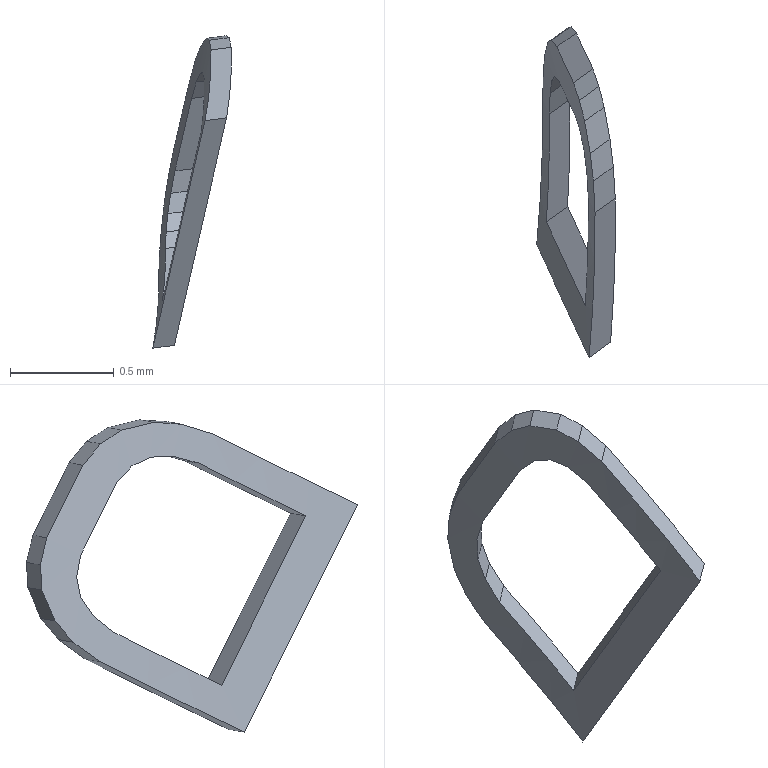Part | SolidWorks | features BaseBody 1 | 1 solid | 28 faces | box 0.379 x 1.595 x 1.505 mm | volume 0.06995 mm3 | plane 26 | cylinder 2 | commonest cylinder face diameters 16.8 x1 17 x1
STEP:
#1=CARTESIAN_POINT('',(1974.698,-243.491,991.242));
#2=VERTEX_POINT('',#1);
#3=CARTESIAN_POINT('',(1974.727,-242.792,991.583));
#4=VERTEX_POINT('',#3);
#5=CARTESIAN_POINT('',(1966.499,-243.608,993.067));
#6=DIRECTION('',(0.2015,-0.436,0.8771));
#7=DIRECTION('',(-0.7309,-0.6631,-0.1618));
#8=AXIS2_PLACEMENT_3D('',#5,#6,#7);
#9=CIRCLE('',#8,8.4);
#10=EDGE_CURVE('',#2,#4,#9,.T.);
#11=ORIENTED_EDGE('',*,*,#10,.T.);
#12=CARTESIAN_POINT('',(1974.718,-242.641,991.629));
#13=VERTEX_POINT('',#12);
#14=CARTESIAN_POINT('',(1974.727,-242.792,991.583));
#15=CARTESIAN_POINT('',(1974.724,-242.742,991.598));
#16=CARTESIAN_POINT('',(1974.722,-242.691,991.614));
#17=CARTESIAN_POINT('',(1974.718,-242.641,991.629));
#18=B_SPLINE_CURVE_WITH_KNOTS('',3,(#14,#15,#16,#17),.UNSPECIFIED.,.F.,.F.,(4,4),(0.,1.),.UNSPECIFIED.);
#19=EDGE_CURVE('',#4,#13,#18,.T.);
#20=ORIENTED_EDGE('',*,*,#19,.T.);
#21=CARTESIAN_POINT('',(1974.704,-242.508,991.638));
#22=VERTEX_POINT('',#21);
#23=CARTESIAN_POINT('',(1974.718,-242.641,991.629));
#24=CARTESIAN_POINT('',(1974.714,-242.597,991.632));
#25=CARTESIAN_POINT('',(1974.709,-242.552,991.635));
#26=CARTESIAN_POINT('',(1974.704,-242.508,991.638));
#27=B_SPLINE_CURVE_WITH_KNOTS('',3,(#23,#24,#25,#26),.UNSPECIFIED.,.F.,.F.,(4,4),(0.,1.),.UNSPECIFIED.);
#28=EDGE_CURVE('',#13,#22,#27,.T.);
#29=ORIENTED_EDGE('',*,*,#28,.T.);
#30=CARTESIAN_POINT('',(1974.676,-242.353,991.6));
#31=VERTEX_POINT('',#30);
#32=CARTESIAN_POINT('',(1974.704,-242.508,991.638));
#33=CARTESIAN_POINT('',(1974.695,-242.456,991.625));
#34=CARTESIAN_POINT('',(1974.686,-242.404,991.613));
#35=CARTESIAN_POINT('',(1974.676,-242.353,991.6));
#36=B_SPLINE_CURVE_WITH_KNOTS('',3,(#32,#33,#34,#35),.UNSPECIFIED.,.F.,.F.,(4,4),(0.,1.),.UNSPECIFIED.);
#37=EDGE_CURVE('',#22,#31,#36,.T.);
#38=ORIENTED_EDGE('',*,*,#37,.T.);
#39=CARTESIAN_POINT('',(1974.651,-242.252,991.534));
#40=VERTEX_POINT('',#39);
#41=CARTESIAN_POINT('',(1974.676,-242.353,991.6));
#42=CARTESIAN_POINT('',(1974.668,-242.319,991.578));
#43=CARTESIAN_POINT('',(1974.66,-242.286,991.556));
#44=CARTESIAN_POINT('',(1974.651,-242.252,991.534));
#45=B_SPLINE_CURVE_WITH_KNOTS('',3,(#41,#42,#43,#44),.UNSPECIFIED.,.F.,.F.,(4,4),(0.,1.),.UNSPECIFIED.);
#46=EDGE_CURVE('',#31,#40,#45,.T.);
#47=ORIENTED_EDGE('',*,*,#46,.T.);
#48=CARTESIAN_POINT('',(1974.623,-242.168,991.432));
#49=VERTEX_POINT('',#48);
#50=CARTESIAN_POINT('',(1974.651,-242.252,991.534));
#51=CARTESIAN_POINT('',(1974.642,-242.224,991.5));
#52=CARTESIAN_POINT('',(1974.632,-242.196,991.466));
#53=CARTESIAN_POINT('',(1974.623,-242.168,991.432));
#54=B_SPLINE_CURVE_WITH_KNOTS('',3,(#50,#51,#52,#53),.UNSPECIFIED.,.F.,.F.,(4,4),(0.,1.),.UNSPECIFIED.);
#55=EDGE_CURVE('',#40,#49,#54,.T.);
#56=ORIENTED_EDGE('',*,*,#55,.T.);
#57=CARTESIAN_POINT('',(1974.542,-241.994,991.082));
#58=VERTEX_POINT('',#57);
#59=CARTESIAN_POINT('',(1975.659,-244.411,995.945));
#60=DIRECTION('',(-0.2015,0.436,-0.8771));
#61=VECTOR('',#60,1000.);
#62=LINE('',#59,#61);
#63=EDGE_CURVE('',#49,#58,#62,.T.);
#64=ORIENTED_EDGE('',*,*,#63,.T.);
#65=CARTESIAN_POINT('',(1974.517,-241.963,990.951));
#66=VERTEX_POINT('',#65);
#67=CARTESIAN_POINT('',(1974.517,-241.963,990.951));
#68=CARTESIAN_POINT('',(1974.526,-241.973,990.995));
#69=CARTESIAN_POINT('',(1974.534,-241.983,991.038));
#70=CARTESIAN_POINT('',(1974.542,-241.994,991.082));
#71=B_SPLINE_CURVE_WITH_KNOTS('',3,(#67,#68,#69,#70),.UNSPECIFIED.,.F.,.F.,(4,4),(0.,1.),.UNSPECIFIED.);
#72=EDGE_CURVE('',#66,#58,#71,.T.);
#73=ORIENTED_EDGE('',*,*,#72,.F.);
#74=CARTESIAN_POINT('',(1974.5,-241.97,990.83));
#75=VERTEX_POINT('',#74);
#76=CARTESIAN_POINT('',(1974.5,-241.97,990.83));
#77=CARTESIAN_POINT('',(1974.506,-241.967,990.871));
#78=CARTESIAN_POINT('',(1974.512,-241.965,990.911));
#79=CARTESIAN_POINT('',(1974.517,-241.963,990.951));
#80=B_SPLINE_CURVE_WITH_KNOTS('',3,(#76,#77,#78,#79),.UNSPECIFIED.,.F.,.F.,(4,4),(0.,1.),.UNSPECIFIED.);
#81=EDGE_CURVE('',#75,#66,#80,.T.);
#82=ORIENTED_EDGE('',*,*,#81,.F.);
#83=CARTESIAN_POINT('',(1974.484,-242.032,990.682));
#84=VERTEX_POINT('',#83);
#85=CARTESIAN_POINT('',(1974.484,-242.032,990.682));
#86=CARTESIAN_POINT('',(1974.489,-242.012,990.731));
#87=CARTESIAN_POINT('',(1974.495,-241.991,990.781));
#88=CARTESIAN_POINT('',(1974.5,-241.97,990.83));
#89=B_SPLINE_CURVE_WITH_KNOTS('',3,(#85,#86,#87,#88),.UNSPECIFIED.,.F.,.F.,(4,4),(0.,1.),.UNSPECIFIED.);
#90=EDGE_CURVE('',#84,#75,#89,.T.);
#91=ORIENTED_EDGE('',*,*,#90,.F.);
#92=CARTESIAN_POINT('',(1974.477,-242.119,990.579));
#93=VERTEX_POINT('',#92);
#94=CARTESIAN_POINT('',(1974.477,-242.119,990.579));
#95=CARTESIAN_POINT('',(1974.48,-242.09,990.613));
#96=CARTESIAN_POINT('',(1974.482,-242.061,990.647));
#97=CARTESIAN_POINT('',(1974.484,-242.032,990.682));
#98=B_SPLINE_CURVE_WITH_KNOTS('',3,(#94,#95,#96,#97),.UNSPECIFIED.,.F.,.F.,(4,4),(0.,1.),.UNSPECIFIED.);
#99=EDGE_CURVE('',#93,#84,#98,.T.);
#100=ORIENTED_EDGE('',*,*,#99,.F.);
#101=CARTESIAN_POINT('',(1974.475,-242.247,990.486));
#102=VERTEX_POINT('',#101);
#103=CARTESIAN_POINT('',(1974.475,-242.247,990.486));
#104=CARTESIAN_POINT('',(1974.476,-242.204,990.517));
#105=CARTESIAN_POINT('',(1974.477,-242.162,990.548));
#106=CARTESIAN_POINT('',(1974.477,-242.119,990.579));
#107=B_SPLINE_CURVE_WITH_KNOTS('',3,(#103,#104,#105,#106),.UNSPECIFIED.,.F.,.F.,(4,4),(0.,1.),.UNSPECIFIED.);
#108=EDGE_CURVE('',#102,#93,#107,.T.);
#109=ORIENTED_EDGE('',*,*,#108,.F.);
#110=CARTESIAN_POINT('',(1974.446,-242.945,990.146));
#111=VERTEX_POINT('',#110);
#112=CARTESIAN_POINT('',(1966.247,-243.063,991.97));
#113=DIRECTION('',(-0.2015,0.436,-0.8771));
#114=DIRECTION('',(-0.7309,-0.6631,-0.1618));
#115=AXIS2_PLACEMENT_3D('',#112,#113,#114);
#116=CIRCLE('',#115,8.4);
#117=EDGE_CURVE('',#102,#111,#116,.T.);
#118=ORIENTED_EDGE('',*,*,#117,.T.);
#119=CARTESIAN_POINT('',(1975.649,-245.549,995.382));
#120=DIRECTION('',(0.2015,-0.436,0.8771));
#121=VECTOR('',#120,1000.);
#122=LINE('',#119,#121);
#123=EDGE_CURVE('',#111,#2,#122,.T.);
#124=ORIENTED_EDGE('',*,*,#123,.T.);
#125=EDGE_LOOP('',(#11,#20,#29,#38,#47,#56,#64,#73,#82,#91,#100,#109,#118,#124));
#126=FACE_OUTER_BOUND('',#125,.T.);
#127=CARTESIAN_POINT('',(1974.507,-242.317,990.626));
#128=VERTEX_POINT('',#127);
#129=CARTESIAN_POINT('',(1974.51,-242.217,990.705));
#130=VERTEX_POINT('',#129);
#131=CARTESIAN_POINT('',(1974.507,-242.317,990.626));
#132=CARTESIAN_POINT('',(1974.508,-242.283,990.652));
#133=CARTESIAN_POINT('',(1974.509,-242.25,990.679));
#134=CARTESIAN_POINT('',(1974.51,-242.217,990.705));
#135=B_SPLINE_CURVE_WITH_KNOTS('',3,(#131,#132,#133,#134),.UNSPECIFIED.,.F.,.F.,(4,4),(0.,1.),.UNSPECIFIED.);
#136=EDGE_CURVE('',#128,#130,#135,.T.);
#137=ORIENTED_EDGE('',*,*,#136,.T.);
#138=CARTESIAN_POINT('',(1974.518,-242.157,990.794));
#139=VERTEX_POINT('',#138);
#140=CARTESIAN_POINT('',(1974.51,-242.217,990.705));
#141=CARTESIAN_POINT('',(1974.513,-242.197,990.735));
#142=CARTESIAN_POINT('',(1974.516,-242.177,990.764));
#143=CARTESIAN_POINT('',(1974.518,-242.157,990.794));
#144=B_SPLINE_CURVE_WITH_KNOTS('',3,(#140,#141,#142,#143),.UNSPECIFIED.,.F.,.F.,(4,4),(0.,1.),.UNSPECIFIED.);
#145=EDGE_CURVE('',#130,#139,#144,.T.);
#146=ORIENTED_EDGE('',*,*,#145,.T.);
#147=CARTESIAN_POINT('',(1974.532,-242.137,990.892));
#148=VERTEX_POINT('',#147);
#149=CARTESIAN_POINT('',(1974.518,-242.157,990.794));
#150=CARTESIAN_POINT('',(1974.523,-242.15,990.826));
#151=CARTESIAN_POINT('',(1974.528,-242.143,990.859));
#152=CARTESIAN_POINT('',(1974.532,-242.137,990.892));
#153=B_SPLINE_CURVE_WITH_KNOTS('',3,(#149,#150,#151,#152),.UNSPECIFIED.,.F.,.F.,(4,4),(0.,1.),.UNSPECIFIED.);
#154=EDGE_CURVE('',#139,#148,#153,.T.);
#155=ORIENTED_EDGE('',*,*,#154,.T.);
#156=CARTESIAN_POINT('',(1974.552,-242.156,990.999));
#157=VERTEX_POINT('',#156);
#158=CARTESIAN_POINT('',(1974.532,-242.137,990.892));
#159=CARTESIAN_POINT('',(1974.539,-242.143,990.927));
#160=CARTESIAN_POINT('',(1974.546,-242.15,990.963));
#161=CARTESIAN_POINT('',(1974.552,-242.156,990.999));
#162=B_SPLINE_CURVE_WITH_KNOTS('',3,(#158,#159,#160,#161),.UNSPECIFIED.,.F.,.F.,(4,4),(0.,1.),.UNSPECIFIED.);
#163=EDGE_CURVE('',#148,#157,#162,.T.);
#164=ORIENTED_EDGE('',*,*,#163,.T.);
#165=CARTESIAN_POINT('',(1974.633,-242.33,991.349));
#166=VERTEX_POINT('',#165);
#167=CARTESIAN_POINT('',(1975.669,-244.574,995.862));
#168=DIRECTION('',(-0.2015,0.436,-0.8771));
#169=VECTOR('',#168,1000.);
#170=LINE('',#167,#169);
#171=EDGE_CURVE('',#166,#157,#170,.T.);
#172=ORIENTED_EDGE('',*,*,#171,.F.);
#173=CARTESIAN_POINT('',(1974.655,-242.404,991.428));
#174=VERTEX_POINT('',#173);
#175=CARTESIAN_POINT('',(1974.655,-242.404,991.428));
#176=CARTESIAN_POINT('',(1974.648,-242.379,991.402));
#177=CARTESIAN_POINT('',(1974.64,-242.354,991.375));
#178=CARTESIAN_POINT('',(1974.633,-242.33,991.349));
#179=B_SPLINE_CURVE_WITH_KNOTS('',3,(#175,#176,#177,#178),.UNSPECIFIED.,.F.,.F.,(4,4),(0.,1.),.UNSPECIFIED.);
#180=EDGE_CURVE('',#174,#166,#179,.T.);
#181=ORIENTED_EDGE('',*,*,#180,.F.);
#182=CARTESIAN_POINT('',(1974.674,-242.493,991.47));
#183=VERTEX_POINT('',#182);
#184=CARTESIAN_POINT('',(1974.674,-242.493,991.47));
#185=CARTESIAN_POINT('',(1974.668,-242.463,991.456));
#186=CARTESIAN_POINT('',(1974.662,-242.433,991.442));
#187=CARTESIAN_POINT('',(1974.655,-242.404,991.428));
#188=B_SPLINE_CURVE_WITH_KNOTS('',3,(#184,#185,#186,#187),.UNSPECIFIED.,.F.,.F.,(4,4),(0.,1.),.UNSPECIFIED.);
#189=EDGE_CURVE('',#183,#174,#188,.T.);
#190=ORIENTED_EDGE('',*,*,#189,.F.);
#191=CARTESIAN_POINT('',(1974.687,-242.599,991.475));
#192=VERTEX_POINT('',#191);
#193=CARTESIAN_POINT('',(1974.687,-242.599,991.475));
#194=CARTESIAN_POINT('',(1974.683,-242.564,991.474));
#195=CARTESIAN_POINT('',(1974.678,-242.529,991.472));
#196=CARTESIAN_POINT('',(1974.674,-242.493,991.47));
#197=B_SPLINE_CURVE_WITH_KNOTS('',3,(#193,#194,#195,#196),.UNSPECIFIED.,.F.,.F.,(4,4),(0.,1.),.UNSPECIFIED.);
#198=EDGE_CURVE('',#192,#183,#197,.T.);
#199=ORIENTED_EDGE('',*,*,#198,.F.);
#200=CARTESIAN_POINT('',(1974.694,-242.722,991.443));
#201=VERTEX_POINT('',#200);
#202=CARTESIAN_POINT('',(1974.694,-242.722,991.443));
#203=CARTESIAN_POINT('',(1974.692,-242.681,991.453));
#204=CARTESIAN_POINT('',(1974.69,-242.64,991.464));
#205=CARTESIAN_POINT('',(1974.687,-242.599,991.475));
#206=B_SPLINE_CURVE_WITH_KNOTS('',3,(#202,#203,#204,#205),.UNSPECIFIED.,.F.,.F.,(4,4),(0.,1.),.UNSPECIFIED.);
#207=EDGE_CURVE('',#201,#192,#206,.T.);
#208=ORIENTED_EDGE('',*,*,#207,.F.);
#209=CARTESIAN_POINT('',(1974.68,-243.241,991.188));
#210=VERTEX_POINT('',#209);
#211=CARTESIAN_POINT('',(1966.467,-243.538,992.927));
#212=DIRECTION('',(0.2015,-0.436,0.8771));
#213=DIRECTION('',(-0.7309,-0.6631,-0.1618));
#214=AXIS2_PLACEMENT_3D('',#211,#212,#213);
#215=CIRCLE('',#214,8.4);
#216=EDGE_CURVE('',#210,#201,#215,.T.);
#217=ORIENTED_EDGE('',*,*,#216,.F.);
#218=CARTESIAN_POINT('',(1974.492,-242.835,990.372));
#219=VERTEX_POINT('',#218);
#220=CARTESIAN_POINT('',(1975.663,-245.369,995.468));
#221=DIRECTION('',(0.2015,-0.436,0.8771));
#222=VECTOR('',#221,1000.);
#223=LINE('',#220,#222);
#224=EDGE_CURVE('',#219,#210,#223,.T.);
#225=ORIENTED_EDGE('',*,*,#224,.F.);
#226=CARTESIAN_POINT('',(1966.279,-243.133,992.11));
#227=DIRECTION('',(-0.2015,0.436,-0.8771));
#228=DIRECTION('',(-0.7309,-0.6631,-0.1618));
#229=AXIS2_PLACEMENT_3D('',#226,#227,#228);
#230=CIRCLE('',#229,8.4);
#231=EDGE_CURVE('',#128,#219,#230,.T.);
#232=ORIENTED_EDGE('',*,*,#231,.F.);
#233=EDGE_LOOP('',(#137,#146,#155,#164,#172,#181,#190,#199,#208,#217,#225,#232));
#234=FACE_BOUND('',#233,.T.);
#235=CARTESIAN_POINT('',(1967.45,-245.666,997.207));
#236=DIRECTION('',(0.2015,-0.436,0.8771));
#237=DIRECTION('',(-0.7309,-0.6631,-0.1618));
#238=AXIS2_PLACEMENT_3D('',#235,#236,#237);
#239=CYLINDRICAL_SURFACE('',#238,8.4);
#240=ADVANCED_FACE('',(#126,#234),#239,.F.);
#241=CARTESIAN_POINT('',(1974.802,-243.416,991.255));
#242=VERTEX_POINT('',#241);
#243=CARTESIAN_POINT('',(1974.75,-243.453,991.248));
#244=DIRECTION('',(-0.8088,-0.5792,-0.1022));
#245=VECTOR('',#244,1000.);
#246=LINE('',#243,#245);
#247=EDGE_CURVE('',#242,#2,#246,.T.);
#248=ORIENTED_EDGE('',*,*,#247,.T.);
#249=ORIENTED_EDGE('',*,*,#123,.F.);
#250=CARTESIAN_POINT('',(1974.55,-242.871,990.159));
#251=VERTEX_POINT('',#250);
#252=CARTESIAN_POINT('',(1974.498,-242.908,990.152));
#253=DIRECTION('',(-0.8088,-0.5792,-0.1022));
#254=VECTOR('',#253,1000.);
#255=LINE('',#252,#254);
#256=EDGE_CURVE('',#251,#111,#255,.T.);
#257=ORIENTED_EDGE('',*,*,#256,.F.);
#258=CARTESIAN_POINT('',(1974.676,-243.144,990.707));
#259=DIRECTION('',(0.2015,-0.436,0.8771));
#260=VECTOR('',#259,1000.);
#261=LINE('',#258,#260);
#262=EDGE_CURVE('',#251,#242,#261,.T.);
#263=ORIENTED_EDGE('',*,*,#262,.T.);
#264=EDGE_LOOP('',(#248,#249,#257,#263));
#265=FACE_OUTER_BOUND('',#264,.T.);
#266=CARTESIAN_POINT('',(1981.31,-238.029,991.013));
#267=DIRECTION('',(0.5526,-0.6888,-0.4693));
#268=DIRECTION('',(-0.2015,0.436,-0.8771));
#269=AXIS2_PLACEMENT_3D('',#266,#267,#268);
#270=PLANE('',#269);
#271=ADVANCED_FACE('',(#265),#270,.T.);
#272=ORIENTED_EDGE('',*,*,#256,.T.);
#273=ORIENTED_EDGE('',*,*,#117,.F.);
#274=CARTESIAN_POINT('',(1974.572,-242.177,990.498));
#275=VERTEX_POINT('',#274);
#276=CARTESIAN_POINT('',(1974.523,-242.212,990.492));
#277=DIRECTION('',(-0.8088,-0.5792,-0.1022));
#278=VECTOR('',#277,1000.);
#279=LINE('',#276,#278);
#280=EDGE_CURVE('',#275,#102,#279,.T.);
#281=ORIENTED_EDGE('',*,*,#280,.F.);
#282=CARTESIAN_POINT('',(1966.247,-243.063,991.97));
#283=DIRECTION('',(-0.2015,0.436,-0.8771));
#284=DIRECTION('',(-0.7309,-0.6631,-0.1618));
#285=AXIS2_PLACEMENT_3D('',#282,#283,#284);
#286=CIRCLE('',#285,8.5);
#287=EDGE_CURVE('',#275,#251,#286,.T.);
#288=ORIENTED_EDGE('',*,*,#287,.T.);
#289=EDGE_LOOP('',(#272,#273,#281,#288));
#290=FACE_OUTER_BOUND('',#289,.T.);
#291=CARTESIAN_POINT('',(1981.656,-238.46,990.719));
#292=DIRECTION('',(-0.2015,0.436,-0.8771));
#293=DIRECTION('',(-0.5526,0.6888,0.4693));
#294=AXIS2_PLACEMENT_3D('',#291,#292,#293);
#295=PLANE('',#294);
#296=ADVANCED_FACE('',(#290),#295,.T.);
#297=ORIENTED_EDGE('',*,*,#280,.T.);
#298=ORIENTED_EDGE('',*,*,#108,.T.);
#299=CARTESIAN_POINT('',(1974.573,-242.051,990.591));
#300=VERTEX_POINT('',#299);
#301=CARTESIAN_POINT('',(1974.525,-242.085,990.585));
#302=DIRECTION('',(-0.8088,-0.5792,-0.1022));
#303=VECTOR('',#302,1000.);
#304=LINE('',#301,#303);
#305=EDGE_CURVE('',#300,#93,#304,.T.);
#306=ORIENTED_EDGE('',*,*,#305,.F.);
#307=CARTESIAN_POINT('',(1974.572,-242.177,990.498));
#308=CARTESIAN_POINT('',(1974.572,-242.152,990.517));
#309=CARTESIAN_POINT('',(1974.573,-242.127,990.536));
#310=CARTESIAN_POINT('',(1974.573,-242.101,990.554));
#311=CARTESIAN_POINT('',(1974.573,-242.076,990.573));
#312=CARTESIAN_POINT('',(1974.573,-242.051,990.591));
#313=B_SPLINE_CURVE_WITH_KNOTS('',5,(#307,#308,#309,#310,#311,#312),.UNSPECIFIED.,.F.,.F.,(6,6),(0.,1.),.UNSPECIFIED.);
#314=EDGE_CURVE('',#275,#300,#313,.T.);
#315=ORIENTED_EDGE('',*,*,#314,.F.);
#316=EDGE_LOOP('',(#297,#298,#306,#315));
#317=FACE_OUTER_BOUND('',#316,.T.);
#318=CARTESIAN_POINT('',(1980.898,-237.521,991.391));
#319=DIRECTION('',(-0.308,0.5651,-0.7654));
#320=DIRECTION('',(-0.5011,0.5876,0.6354));
#321=AXIS2_PLACEMENT_3D('',#318,#319,#320);
#322=PLANE('',#321);
#323=ADVANCED_FACE('',(#317),#322,.T.);
#324=ORIENTED_EDGE('',*,*,#305,.T.);
#325=ORIENTED_EDGE('',*,*,#99,.T.);
#326=CARTESIAN_POINT('',(1974.579,-241.964,990.694));
#327=VERTEX_POINT('',#326);
#328=CARTESIAN_POINT('',(1974.531,-241.998,990.688));
#329=DIRECTION('',(-0.8088,-0.5792,-0.1022));
#330=VECTOR('',#329,1000.);
#331=LINE('',#328,#330);
#332=EDGE_CURVE('',#327,#84,#331,.T.);
#333=ORIENTED_EDGE('',*,*,#332,.F.);
#334=CARTESIAN_POINT('',(1974.573,-242.051,990.591));
#335=CARTESIAN_POINT('',(1974.575,-242.033,990.612));
#336=CARTESIAN_POINT('',(1974.576,-242.016,990.632));
#337=CARTESIAN_POINT('',(1974.577,-241.999,990.653));
#338=CARTESIAN_POINT('',(1974.578,-241.982,990.673));
#339=CARTESIAN_POINT('',(1974.579,-241.964,990.694));
#340=B_SPLINE_CURVE_WITH_KNOTS('',5,(#334,#335,#336,#337,#338,#339),.UNSPECIFIED.,.F.,.F.,(6,6),(0.,1.),.UNSPECIFIED.);
#341=EDGE_CURVE('',#300,#327,#340,.T.);
#342=ORIENTED_EDGE('',*,*,#341,.F.);
#343=EDGE_LOOP('',(#324,#325,#333,#342));
#344=FACE_OUTER_BOUND('',#343,.T.);
#345=CARTESIAN_POINT('',(1980.851,-237.472,991.486));
#346=DIRECTION('',(-0.4307,0.7016,-0.5677));
#347=DIRECTION('',(-0.4005,0.4151,0.8169));
#348=AXIS2_PLACEMENT_3D('',#345,#346,#347);
#349=PLANE('',#348);
#350=ADVANCED_FACE('',(#344),#349,.T.);
#351=ORIENTED_EDGE('',*,*,#332,.T.);
#352=ORIENTED_EDGE('',*,*,#90,.T.);
#353=CARTESIAN_POINT('',(1974.594,-241.903,990.842));
#354=VERTEX_POINT('',#353);
#355=CARTESIAN_POINT('',(1974.547,-241.936,990.836));
#356=DIRECTION('',(-0.8088,-0.5792,-0.1022));
#357=VECTOR('',#356,1000.);
#358=LINE('',#355,#357);
#359=EDGE_CURVE('',#354,#75,#358,.T.);
#360=ORIENTED_EDGE('',*,*,#359,.F.);
#361=CARTESIAN_POINT('',(1974.579,-241.964,990.694));
#362=CARTESIAN_POINT('',(1974.582,-241.952,990.723));
#363=CARTESIAN_POINT('',(1974.585,-241.939,990.753));
#364=CARTESIAN_POINT('',(1974.588,-241.927,990.783));
#365=CARTESIAN_POINT('',(1974.591,-241.915,990.813));
#366=CARTESIAN_POINT('',(1974.594,-241.903,990.842));
#367=B_SPLINE_CURVE_WITH_KNOTS('',5,(#361,#362,#363,#364,#365,#366),.UNSPECIFIED.,.F.,.F.,(6,6),(0.,1.),.UNSPECIFIED.);
#368=EDGE_CURVE('',#327,#354,#367,.T.);
#369=ORIENTED_EDGE('',*,*,#368,.F.);
#370=EDGE_LOOP('',(#351,#352,#360,#369));
#371=FACE_OUTER_BOUND('',#370,.T.);
#372=CARTESIAN_POINT('',(1980.815,-237.447,991.628));
#373=DIRECTION('',(-0.5358,0.7972,-0.2783));
#374=DIRECTION('',(-0.2426,0.1703,0.955));
#375=AXIS2_PLACEMENT_3D('',#372,#373,#374);
#376=PLANE('',#375);
#377=ADVANCED_FACE('',(#371),#376,.T.);
#378=ORIENTED_EDGE('',*,*,#359,.T.);
#379=ORIENTED_EDGE('',*,*,#81,.T.);
#380=CARTESIAN_POINT('',(1974.611,-241.895,990.963));
#381=VERTEX_POINT('',#380);
#382=CARTESIAN_POINT('',(1974.564,-241.929,990.957));
#383=DIRECTION('',(-0.8088,-0.5792,-0.1022));
#384=VECTOR('',#383,1000.);
#385=LINE('',#382,#384);
#386=EDGE_CURVE('',#381,#66,#385,.T.);
#387=ORIENTED_EDGE('',*,*,#386,.F.);
#388=CARTESIAN_POINT('',(1974.594,-241.903,990.842));
#389=CARTESIAN_POINT('',(1974.597,-241.901,990.866));
#390=CARTESIAN_POINT('',(1974.601,-241.9,990.891));
#391=CARTESIAN_POINT('',(1974.604,-241.898,990.915));
#392=CARTESIAN_POINT('',(1974.608,-241.897,990.939));
#393=CARTESIAN_POINT('',(1974.611,-241.895,990.963));
#394=B_SPLINE_CURVE_WITH_KNOTS('',5,(#388,#389,#390,#391,#392,#393),.UNSPECIFIED.,.F.,.F.,(6,6),(0.,1.),.UNSPECIFIED.);
#395=EDGE_CURVE('',#354,#381,#394,.T.);
#396=ORIENTED_EDGE('',*,*,#395,.F.);
#397=EDGE_LOOP('',(#378,#379,#387,#396));
#398=FACE_OUTER_BOUND('',#397,.T.);
#399=CARTESIAN_POINT('',(1980.808,-237.457,991.746));
#400=DIRECTION('',(-0.5849,0.8103,0.03586));
#401=DIRECTION('',(-0.06203,-0.08877,0.9941));
#402=AXIS2_PLACEMENT_3D('',#399,#400,#401);
#403=PLANE('',#402);
#404=ADVANCED_FACE('',(#398),#403,.T.);
#405=ORIENTED_EDGE('',*,*,#386,.T.);
#406=ORIENTED_EDGE('',*,*,#72,.T.);
#407=CARTESIAN_POINT('',(1974.636,-241.927,991.094));
#408=VERTEX_POINT('',#407);
#409=CARTESIAN_POINT('',(1974.589,-241.96,991.088));
#410=DIRECTION('',(-0.8088,-0.5792,-0.1022));
#411=VECTOR('',#410,1000.);
#412=LINE('',#409,#411);
#413=EDGE_CURVE('',#408,#58,#412,.T.);
#414=ORIENTED_EDGE('',*,*,#413,.F.);
#415=CARTESIAN_POINT('',(1974.611,-241.895,990.963));
#416=CARTESIAN_POINT('',(1974.616,-241.902,990.989));
#417=CARTESIAN_POINT('',(1974.621,-241.908,991.015));
#418=CARTESIAN_POINT('',(1974.626,-241.914,991.041));
#419=CARTESIAN_POINT('',(1974.631,-241.92,991.068));
#420=CARTESIAN_POINT('',(1974.636,-241.927,991.094));
#421=B_SPLINE_CURVE_WITH_KNOTS('',5,(#415,#416,#417,#418,#419,#420),.UNSPECIFIED.,.F.,.F.,(6,6),(0.,1.),.UNSPECIFIED.);
#422=EDGE_CURVE('',#381,#408,#421,.T.);
#423=ORIENTED_EDGE('',*,*,#422,.F.);
#424=EDGE_LOOP('',(#405,#406,#414,#423));
#425=FACE_OUTER_BOUND('',#424,.T.);
#426=CARTESIAN_POINT('',(1980.82,-237.497,991.875));
#427=DIRECTION('',(-0.581,0.7597,0.292));
#428=DIRECTION('',(0.09152,-0.2955,0.9509));
#429=AXIS2_PLACEMENT_3D('',#426,#427,#428);
#430=PLANE('',#429);
#431=ADVANCED_FACE('',(#425),#430,.T.);
#432=ORIENTED_EDGE('',*,*,#413,.T.);
#433=ORIENTED_EDGE('',*,*,#63,.F.);
#434=CARTESIAN_POINT('',(1974.716,-242.1,991.443));
#435=VERTEX_POINT('',#434);
#436=CARTESIAN_POINT('',(1974.669,-242.134,991.438));
#437=DIRECTION('',(-0.8088,-0.5792,-0.1022));
#438=VECTOR('',#437,1000.);
#439=LINE('',#436,#438);
#440=EDGE_CURVE('',#435,#49,#439,.T.);
#441=ORIENTED_EDGE('',*,*,#440,.F.);
#442=CARTESIAN_POINT('',(1974.676,-242.014,991.269));
#443=DIRECTION('',(-0.2015,0.436,-0.8771));
#444=VECTOR('',#443,1000.);
#445=LINE('',#442,#444);
#446=EDGE_CURVE('',#435,#408,#445,.T.);
#447=ORIENTED_EDGE('',*,*,#446,.T.);
#448=EDGE_LOOP('',(#432,#433,#441,#447));
#449=FACE_OUTER_BOUND('',#448,.T.);
#450=CARTESIAN_POINT('',(1980.901,-237.671,992.225));
#451=DIRECTION('',(-0.5526,0.6888,0.4693));
#452=DIRECTION('',(0.2015,-0.436,0.8771));
#453=AXIS2_PLACEMENT_3D('',#450,#451,#452);
#454=PLANE('',#453);
#455=ADVANCED_FACE('',(#449),#454,.T.);
#456=ORIENTED_EDGE('',*,*,#440,.T.);
#457=ORIENTED_EDGE('',*,*,#55,.F.);
#458=CARTESIAN_POINT('',(1974.745,-242.185,991.546));
#459=VERTEX_POINT('',#458);
#460=CARTESIAN_POINT('',(1974.698,-242.219,991.54));
#461=DIRECTION('',(-0.8088,-0.5792,-0.1022));
#462=VECTOR('',#461,1000.);
#463=LINE('',#460,#462);
#464=EDGE_CURVE('',#459,#40,#463,.T.);
#465=ORIENTED_EDGE('',*,*,#464,.F.);
#466=CARTESIAN_POINT('',(1974.745,-242.185,991.546));
#467=CARTESIAN_POINT('',(1974.739,-242.168,991.526));
#468=CARTESIAN_POINT('',(1974.734,-242.151,991.505));
#469=CARTESIAN_POINT('',(1974.728,-242.134,991.485));
#470=CARTESIAN_POINT('',(1974.722,-242.117,991.464));
#471=CARTESIAN_POINT('',(1974.716,-242.1,991.443));
#472=B_SPLINE_CURVE_WITH_KNOTS('',5,(#466,#467,#468,#469,#470,#471),.UNSPECIFIED.,.F.,.F.,(6,6),(0.,1.),.UNSPECIFIED.);
#473=EDGE_CURVE('',#459,#435,#472,.T.);
#474=ORIENTED_EDGE('',*,*,#473,.T.);
#475=EDGE_LOOP('',(#456,#457,#465,#474));
#476=FACE_OUTER_BOUND('',#475,.T.);
#477=CARTESIAN_POINT('',(1980.942,-237.747,992.329));
#478=DIRECTION('',(-0.5035,0.5921,0.6292));
#479=DIRECTION('',(0.3039,-0.5603,0.7705));
#480=AXIS2_PLACEMENT_3D('',#477,#478,#479);
#481=PLANE('',#480);
#482=ADVANCED_FACE('',(#476),#481,.T.);
#483=ORIENTED_EDGE('',*,*,#464,.T.);
#484=ORIENTED_EDGE('',*,*,#46,.F.);
#485=CARTESIAN_POINT('',(1974.771,-242.285,991.612));
#486=VERTEX_POINT('',#485);
#487=CARTESIAN_POINT('',(1974.723,-242.319,991.606));
#488=DIRECTION('',(-0.8088,-0.5792,-0.1022));
#489=VECTOR('',#488,1000.);
#490=LINE('',#487,#489);
#491=EDGE_CURVE('',#486,#31,#490,.T.);
#492=ORIENTED_EDGE('',*,*,#491,.F.);
#493=CARTESIAN_POINT('',(1974.771,-242.285,991.612));
#494=CARTESIAN_POINT('',(1974.766,-242.265,991.599));
#495=CARTESIAN_POINT('',(1974.761,-242.245,991.586));
#496=CARTESIAN_POINT('',(1974.755,-242.225,991.573));
#497=CARTESIAN_POINT('',(1974.75,-242.205,991.56));
#498=CARTESIAN_POINT('',(1974.745,-242.185,991.546));
#499=B_SPLINE_CURVE_WITH_KNOTS('',5,(#493,#494,#495,#496,#497,#498),.UNSPECIFIED.,.F.,.F.,(6,6),(0.,1.),.UNSPECIFIED.);
#500=EDGE_CURVE('',#486,#459,#499,.T.);
#501=ORIENTED_EDGE('',*,*,#500,.T.);
#502=EDGE_LOOP('',(#483,#484,#492,#501));
#503=FACE_OUTER_BOUND('',#502,.T.);
#504=CARTESIAN_POINT('',(1980.992,-237.83,992.398));
#505=DIRECTION('',(-0.4077,0.4269,0.8072));
#506=DIRECTION('',(0.4239,-0.6945,0.5814));
#507=AXIS2_PLACEMENT_3D('',#504,#505,#506);
#508=PLANE('',#507);
#509=ADVANCED_FACE('',(#503),#508,.T.);
#510=ORIENTED_EDGE('',*,*,#491,.T.);
#511=ORIENTED_EDGE('',*,*,#37,.F.);
#512=CARTESIAN_POINT('',(1974.799,-242.44,991.65));
#513=VERTEX_POINT('',#512);
#514=CARTESIAN_POINT('',(1974.751,-242.474,991.644));
#515=DIRECTION('',(-0.8088,-0.5792,-0.1022));
#516=VECTOR('',#515,1000.);
#517=LINE('',#514,#516);
#518=EDGE_CURVE('',#513,#22,#517,.T.);
#519=ORIENTED_EDGE('',*,*,#518,.F.);
#520=CARTESIAN_POINT('',(1974.799,-242.44,991.65));
#521=CARTESIAN_POINT('',(1974.793,-242.409,991.643));
#522=CARTESIAN_POINT('',(1974.788,-242.378,991.635));
#523=CARTESIAN_POINT('',(1974.782,-242.347,991.627));
#524=CARTESIAN_POINT('',(1974.776,-242.316,991.62));
#525=CARTESIAN_POINT('',(1974.771,-242.285,991.612));
#526=B_SPLINE_CURVE_WITH_KNOTS('',5,(#520,#521,#522,#523,#524,#525),.UNSPECIFIED.,.F.,.F.,(6,6),(0.,1.),.UNSPECIFIED.);
#527=EDGE_CURVE('',#513,#486,#526,.T.);
#528=ORIENTED_EDGE('',*,*,#527,.T.);
#529=EDGE_LOOP('',(#510,#511,#519,#528));
#530=FACE_OUTER_BOUND('',#529,.T.);
#531=CARTESIAN_POINT('',(1981.071,-237.948,992.443));
#532=DIRECTION('',(-0.2539,0.1871,0.949));
#533=DIRECTION('',(0.5305,-0.7934,0.2983));
#534=AXIS2_PLACEMENT_3D('',#531,#532,#533);
#535=PLANE('',#534);
#536=ADVANCED_FACE('',(#530),#535,.T.);
#537=ORIENTED_EDGE('',*,*,#518,.T.);
#538=ORIENTED_EDGE('',*,*,#28,.F.);
#539=CARTESIAN_POINT('',(1974.814,-242.572,991.641));
#540=VERTEX_POINT('',#539);
#541=CARTESIAN_POINT('',(1974.766,-242.607,991.635));
#542=DIRECTION('',(-0.8088,-0.5792,-0.1022));
#543=VECTOR('',#542,1000.);
#544=LINE('',#541,#543);
#545=EDGE_CURVE('',#540,#13,#544,.T.);
#546=ORIENTED_EDGE('',*,*,#545,.F.);
#547=CARTESIAN_POINT('',(1974.814,-242.572,991.641));
#548=CARTESIAN_POINT('',(1974.811,-242.546,991.643));
#549=CARTESIAN_POINT('',(1974.808,-242.519,991.645));
#550=CARTESIAN_POINT('',(1974.805,-242.493,991.647));
#551=CARTESIAN_POINT('',(1974.802,-242.466,991.648));
#552=CARTESIAN_POINT('',(1974.799,-242.44,991.65));
#553=B_SPLINE_CURVE_WITH_KNOTS('',5,(#547,#548,#549,#550,#551,#552),.UNSPECIFIED.,.F.,.F.,(6,6),(0.,1.),.UNSPECIFIED.);
#554=EDGE_CURVE('',#540,#513,#553,.T.);
#555=ORIENTED_EDGE('',*,*,#554,.T.);
#556=EDGE_LOOP('',(#537,#538,#546,#555));
#557=FACE_OUTER_BOUND('',#556,.T.);
#558=CARTESIAN_POINT('',(1981.139,-238.043,992.44));
#559=DIRECTION('',(-0.07187,-0.07511,0.9946));
#560=DIRECTION('',(0.5837,-0.8117,-0.01912));
#561=AXIS2_PLACEMENT_3D('',#558,#559,#560);
#562=PLANE('',#561);
#563=ADVANCED_FACE('',(#557),#562,.T.);
#564=ORIENTED_EDGE('',*,*,#545,.T.);
#565=ORIENTED_EDGE('',*,*,#19,.F.);
#566=CARTESIAN_POINT('',(1974.824,-242.722,991.595));
#567=VERTEX_POINT('',#566);
#568=CARTESIAN_POINT('',(1974.775,-242.757,991.589));
#569=DIRECTION('',(-0.8088,-0.5792,-0.1022));
#570=VECTOR('',#569,1000.);
#571=LINE('',#568,#570);
#572=EDGE_CURVE('',#567,#4,#571,.T.);
#573=ORIENTED_EDGE('',*,*,#572,.F.);
#574=CARTESIAN_POINT('',(1974.824,-242.722,991.595));
#575=CARTESIAN_POINT('',(1974.822,-242.692,991.604));
#576=CARTESIAN_POINT('',(1974.82,-242.662,991.613));
#577=CARTESIAN_POINT('',(1974.819,-242.632,991.623));
#578=CARTESIAN_POINT('',(1974.817,-242.602,991.632));
#579=CARTESIAN_POINT('',(1974.814,-242.572,991.641));
#580=B_SPLINE_CURVE_WITH_KNOTS('',5,(#574,#575,#576,#577,#578,#579),.UNSPECIFIED.,.F.,.F.,(6,6),(0.,1.),.UNSPECIFIED.);
#581=EDGE_CURVE('',#567,#540,#580,.T.);
#582=ORIENTED_EDGE('',*,*,#581,.T.);
#583=EDGE_LOOP('',(#564,#565,#573,#582));
#584=FACE_OUTER_BOUND('',#583,.T.);
#585=CARTESIAN_POINT('',(1981.217,-238.144,992.403));
#586=DIRECTION('',(0.08681,-0.2894,0.9533));
#587=DIRECTION('',(0.5817,-0.7621,-0.2843));
#588=AXIS2_PLACEMENT_3D('',#585,#586,#587);
#589=PLANE('',#588);
#590=ADVANCED_FACE('',(#584),#589,.T.);
#591=ORIENTED_EDGE('',*,*,#572,.T.);
#592=ORIENTED_EDGE('',*,*,#10,.F.);
#593=ORIENTED_EDGE('',*,*,#247,.F.);
#594=CARTESIAN_POINT('',(1966.499,-243.608,993.067));
#595=DIRECTION('',(0.2015,-0.436,0.8771));
#596=DIRECTION('',(-0.7309,-0.6631,-0.1618));
#597=AXIS2_PLACEMENT_3D('',#594,#595,#596);
#598=CIRCLE('',#597,8.5);
#599=EDGE_CURVE('',#242,#567,#598,.T.);
#600=ORIENTED_EDGE('',*,*,#599,.T.);
#601=EDGE_LOOP('',(#591,#592,#593,#600));
#602=FACE_OUTER_BOUND('',#601,.T.);
#603=CARTESIAN_POINT('',(1982.253,-239.435,991.522));
#604=DIRECTION('',(0.2015,-0.436,0.8771));
#605=DIRECTION('',(0.5526,-0.6888,-0.4693));
#606=AXIS2_PLACEMENT_3D('',#603,#604,#605);
#607=PLANE('',#606);
#608=ADVANCED_FACE('',(#602),#607,.T.);
#609=CARTESIAN_POINT('',(1974.604,-242.247,990.638));
#610=VERTEX_POINT('',#609);
#611=CARTESIAN_POINT('',(1974.594,-242.762,990.384));
#612=VERTEX_POINT('',#611);
#613=CARTESIAN_POINT('',(1966.279,-243.133,992.11));
#614=DIRECTION('',(-0.2015,0.436,-0.8771));
#615=DIRECTION('',(-0.7309,-0.6631,-0.1618));
#616=AXIS2_PLACEMENT_3D('',#613,#614,#615);
#617=CIRCLE('',#616,8.5);
#618=EDGE_CURVE('',#610,#612,#617,.T.);
#619=ORIENTED_EDGE('',*,*,#618,.F.);
#620=CARTESIAN_POINT('',(1974.555,-242.282,990.632));
#621=DIRECTION('',(-0.8088,-0.5792,-0.1022));
#622=VECTOR('',#621,1000.);
#623=LINE('',#620,#622);
#624=EDGE_CURVE('',#610,#128,#623,.T.);
#625=ORIENTED_EDGE('',*,*,#624,.T.);
#626=ORIENTED_EDGE('',*,*,#231,.T.);
#627=CARTESIAN_POINT('',(1974.543,-242.799,990.378));
#628=DIRECTION('',(-0.8088,-0.5792,-0.1022));
#629=VECTOR('',#628,1000.);
#630=LINE('',#627,#629);
#631=EDGE_CURVE('',#612,#219,#630,.T.);
#632=ORIENTED_EDGE('',*,*,#631,.F.);
#633=EDGE_LOOP('',(#619,#625,#626,#632));
#634=FACE_OUTER_BOUND('',#633,.T.);
#635=CARTESIAN_POINT('',(1981.688,-238.529,990.859));
#636=DIRECTION('',(-0.2015,0.436,-0.8771));
#637=DIRECTION('',(-0.5526,0.6888,0.4693));
#638=AXIS2_PLACEMENT_3D('',#635,#636,#637);
#639=PLANE('',#638);
#640=ADVANCED_FACE('',(#634),#639,.F.);
#641=CARTESIAN_POINT('',(1974.782,-243.168,991.201));
#642=VERTEX_POINT('',#641);
#643=CARTESIAN_POINT('',(1974.688,-242.965,990.793));
#644=DIRECTION('',(0.2015,-0.436,0.8771));
#645=VECTOR('',#644,1000.);
#646=LINE('',#643,#645);
#647=EDGE_CURVE('',#612,#642,#646,.T.);
#648=ORIENTED_EDGE('',*,*,#647,.F.);
#649=ORIENTED_EDGE('',*,*,#631,.T.);
#650=ORIENTED_EDGE('',*,*,#224,.T.);
#651=CARTESIAN_POINT('',(1974.731,-243.205,991.194));
#652=DIRECTION('',(-0.8088,-0.5792,-0.1022));
#653=VECTOR('',#652,1000.);
#654=LINE('',#651,#653);
#655=EDGE_CURVE('',#642,#210,#654,.T.);
#656=ORIENTED_EDGE('',*,*,#655,.F.);
#657=EDGE_LOOP('',(#648,#649,#650,#656));
#658=FACE_OUTER_BOUND('',#657,.T.);
#659=CARTESIAN_POINT('',(1981.256,-237.991,991.226));
#660=DIRECTION('',(0.5526,-0.6888,-0.4693));
#661=DIRECTION('',(-0.2015,0.436,-0.8771));
#662=AXIS2_PLACEMENT_3D('',#659,#660,#661);
#663=PLANE('',#662);
#664=ADVANCED_FACE('',(#658),#663,.F.);
#665=CARTESIAN_POINT('',(1974.792,-242.653,991.455));
#666=VERTEX_POINT('',#665);
#667=CARTESIAN_POINT('',(1966.467,-243.538,992.927));
#668=DIRECTION('',(0.2015,-0.436,0.8771));
#669=DIRECTION('',(-0.7309,-0.6631,-0.1618));
#670=AXIS2_PLACEMENT_3D('',#667,#668,#669);
#671=CIRCLE('',#670,8.5);
#672=EDGE_CURVE('',#642,#666,#671,.T.);
#673=ORIENTED_EDGE('',*,*,#672,.F.);
#674=ORIENTED_EDGE('',*,*,#655,.T.);
#675=ORIENTED_EDGE('',*,*,#216,.T.);
#676=CARTESIAN_POINT('',(1974.743,-242.688,991.449));
#677=DIRECTION('',(-0.8088,-0.5792,-0.1022));
#678=VECTOR('',#677,1000.);
#679=LINE('',#676,#678);
#680=EDGE_CURVE('',#666,#201,#679,.T.);
#681=ORIENTED_EDGE('',*,*,#680,.F.);
#682=EDGE_LOOP('',(#673,#674,#675,#681));
#683=FACE_OUTER_BOUND('',#682,.T.);
#684=CARTESIAN_POINT('',(1982.134,-239.258,991.456));
#685=DIRECTION('',(0.2015,-0.436,0.8771));
#686=DIRECTION('',(0.5526,-0.6888,-0.4693));
#687=AXIS2_PLACEMENT_3D('',#684,#685,#686);
#688=PLANE('',#687);
#689=ADVANCED_FACE('',(#683),#688,.F.);
#690=CARTESIAN_POINT('',(1974.783,-242.53,991.487));
#691=VERTEX_POINT('',#690);
#692=CARTESIAN_POINT('',(1974.792,-242.653,991.455));
#693=CARTESIAN_POINT('',(1974.79,-242.628,991.461));
#694=CARTESIAN_POINT('',(1974.789,-242.604,991.468));
#695=CARTESIAN_POINT('',(1974.787,-242.579,991.474));
#696=CARTESIAN_POINT('',(1974.785,-242.555,991.481));
#697=CARTESIAN_POINT('',(1974.783,-242.53,991.487));
#698=B_SPLINE_CURVE_WITH_KNOTS('',5,(#692,#693,#694,#695,#696,#697),.UNSPECIFIED.,.F.,.F.,(6,6),(0.,1.),.UNSPECIFIED.);
#699=EDGE_CURVE('',#666,#691,#698,.T.);
#700=ORIENTED_EDGE('',*,*,#699,.F.);
#701=ORIENTED_EDGE('',*,*,#680,.T.);
#702=ORIENTED_EDGE('',*,*,#207,.T.);
#703=CARTESIAN_POINT('',(1974.735,-242.565,991.481));
#704=DIRECTION('',(-0.8088,-0.5792,-0.1022));
#705=VECTOR('',#704,1000.);
#706=LINE('',#703,#705);
#707=EDGE_CURVE('',#691,#192,#706,.T.);
#708=ORIENTED_EDGE('',*,*,#707,.F.);
#709=EDGE_LOOP('',(#700,#701,#702,#708));
#710=FACE_OUTER_BOUND('',#709,.T.);
#711=CARTESIAN_POINT('',(1981.185,-238.074,992.263));
#712=DIRECTION('',(0.05851,-0.2521,0.9659));
#713=DIRECTION('',(0.5852,-0.7752,-0.2378));
#714=AXIS2_PLACEMENT_3D('',#711,#712,#713);
#715=PLANE('',#714);
#716=ADVANCED_FACE('',(#710),#715,.F.);
#717=CARTESIAN_POINT('',(1974.769,-242.425,991.482));
#718=VERTEX_POINT('',#717);
#719=CARTESIAN_POINT('',(1974.783,-242.53,991.487));
#720=CARTESIAN_POINT('',(1974.781,-242.509,991.486));
#721=CARTESIAN_POINT('',(1974.778,-242.488,991.485));
#722=CARTESIAN_POINT('',(1974.775,-242.467,991.484));
#723=CARTESIAN_POINT('',(1974.772,-242.446,991.483));
#724=CARTESIAN_POINT('',(1974.769,-242.425,991.482));
#725=B_SPLINE_CURVE_WITH_KNOTS('',5,(#719,#720,#721,#722,#723,#724),.UNSPECIFIED.,.F.,.F.,(6,6),(0.,1.),.UNSPECIFIED.);
#726=EDGE_CURVE('',#691,#718,#725,.T.);
#727=ORIENTED_EDGE('',*,*,#726,.F.);
#728=ORIENTED_EDGE('',*,*,#707,.T.);
#729=ORIENTED_EDGE('',*,*,#198,.T.);
#730=CARTESIAN_POINT('',(1974.722,-242.459,991.476));
#731=DIRECTION('',(-0.8088,-0.5792,-0.1022));
#732=VECTOR('',#731,1000.);
#733=LINE('',#730,#732);
#734=EDGE_CURVE('',#718,#183,#733,.T.);
#735=ORIENTED_EDGE('',*,*,#734,.F.);
#736=EDGE_LOOP('',(#727,#728,#729,#735));
#737=FACE_OUTER_BOUND('',#736,.T.);
#738=CARTESIAN_POINT('',(1981.122,-237.991,992.288));
#739=DIRECTION('',(-0.1444,0.0272,0.9891));
#740=DIRECTION('',(0.5701,-0.8147,0.1057));
#741=AXIS2_PLACEMENT_3D('',#738,#739,#740);
#742=PLANE('',#741);
#743=ADVANCED_FACE('',(#737),#742,.F.);
#744=CARTESIAN_POINT('',(1974.751,-242.335,991.44));
#745=VERTEX_POINT('',#744);
#746=CARTESIAN_POINT('',(1974.769,-242.425,991.482));
#747=CARTESIAN_POINT('',(1974.766,-242.407,991.474));
#748=CARTESIAN_POINT('',(1974.762,-242.389,991.465));
#749=CARTESIAN_POINT('',(1974.758,-242.371,991.457));
#750=CARTESIAN_POINT('',(1974.754,-242.353,991.449));
#751=CARTESIAN_POINT('',(1974.751,-242.335,991.44));
#752=B_SPLINE_CURVE_WITH_KNOTS('',5,(#746,#747,#748,#749,#750,#751),.UNSPECIFIED.,.F.,.F.,(6,6),(0.,1.),.UNSPECIFIED.);
#753=EDGE_CURVE('',#718,#745,#752,.T.);
#754=ORIENTED_EDGE('',*,*,#753,.F.);
#755=ORIENTED_EDGE('',*,*,#734,.T.);
#756=ORIENTED_EDGE('',*,*,#189,.T.);
#757=CARTESIAN_POINT('',(1974.703,-242.369,991.434));
#758=DIRECTION('',(-0.8088,-0.5792,-0.1022));
#759=VECTOR('',#758,1000.);
#760=LINE('',#757,#759);
#761=EDGE_CURVE('',#745,#174,#760,.T.);
#762=ORIENTED_EDGE('',*,*,#761,.F.);
#763=EDGE_LOOP('',(#754,#755,#756,#762));
#764=FACE_OUTER_BOUND('',#763,.T.);
#765=CARTESIAN_POINT('',(1981.068,-237.914,992.278));
#766=DIRECTION('',(-0.3526,0.3384,0.8724));
#767=DIRECTION('',(0.4707,-0.7416,0.4779));
#768=AXIS2_PLACEMENT_3D('',#765,#766,#767);
#769=PLANE('',#768);
#770=ADVANCED_FACE('',(#764),#769,.F.);
#771=CARTESIAN_POINT('',(1974.728,-242.262,991.361));
#772=VERTEX_POINT('',#771);
#773=CARTESIAN_POINT('',(1974.751,-242.335,991.44));
#774=CARTESIAN_POINT('',(1974.746,-242.321,991.424));
#775=CARTESIAN_POINT('',(1974.741,-242.306,991.408));
#776=CARTESIAN_POINT('',(1974.737,-242.291,991.392));
#777=CARTESIAN_POINT('',(1974.732,-242.277,991.377));
#778=CARTESIAN_POINT('',(1974.728,-242.262,991.361));
#779=B_SPLINE_CURVE_WITH_KNOTS('',5,(#773,#774,#775,#776,#777,#778),.UNSPECIFIED.,.F.,.F.,(6,6),(0.,1.),.UNSPECIFIED.);
#780=EDGE_CURVE('',#745,#772,#779,.T.);
#781=ORIENTED_EDGE('',*,*,#780,.F.);
#782=ORIENTED_EDGE('',*,*,#761,.T.);
#783=ORIENTED_EDGE('',*,*,#180,.T.);
#784=CARTESIAN_POINT('',(1974.68,-242.296,991.355));
#785=DIRECTION('',(-0.8088,-0.5792,-0.1022));
#786=VECTOR('',#785,1000.);
#787=LINE('',#784,#786);
#788=EDGE_CURVE('',#772,#166,#787,.T.);
#789=ORIENTED_EDGE('',*,*,#788,.F.);
#790=EDGE_LOOP('',(#781,#782,#783,#789));
#791=FACE_OUTER_BOUND('',#790,.T.);
#792=CARTESIAN_POINT('',(1981.023,-237.843,992.233));
#793=DIRECTION('',(-0.4888,0.5653,0.6644));
#794=DIRECTION('',(0.3271,-0.5873,0.7403));
#795=AXIS2_PLACEMENT_3D('',#792,#793,#794);
#796=PLANE('',#795);
#797=ADVANCED_FACE('',(#791),#796,.F.);
#798=CARTESIAN_POINT('',(1974.647,-242.088,991.011));
#799=VERTEX_POINT('',#798);
#800=CARTESIAN_POINT('',(1974.687,-242.175,991.186));
#801=DIRECTION('',(-0.2015,0.436,-0.8771));
#802=VECTOR('',#801,1000.);
#803=LINE('',#800,#802);
#804=EDGE_CURVE('',#772,#799,#803,.T.);
#805=ORIENTED_EDGE('',*,*,#804,.F.);
#806=ORIENTED_EDGE('',*,*,#788,.T.);
#807=ORIENTED_EDGE('',*,*,#171,.T.);
#808=CARTESIAN_POINT('',(1974.6,-242.122,991.005));
#809=DIRECTION('',(-0.8088,-0.5792,-0.1022));
#810=VECTOR('',#809,1000.);
#811=LINE('',#808,#810);
#812=EDGE_CURVE('',#799,#157,#811,.T.);
#813=ORIENTED_EDGE('',*,*,#812,.F.);
#814=EDGE_LOOP('',(#805,#806,#807,#813));
#815=FACE_OUTER_BOUND('',#814,.T.);
#816=CARTESIAN_POINT('',(1980.987,-237.779,992.151));
#817=DIRECTION('',(-0.5526,0.6888,0.4693));
#818=DIRECTION('',(0.2015,-0.436,0.8771));
#819=AXIS2_PLACEMENT_3D('',#816,#817,#818);
#820=PLANE('',#819);
#821=ADVANCED_FACE('',(#815),#820,.F.);
#822=CARTESIAN_POINT('',(1974.627,-242.069,990.904));
#823=VERTEX_POINT('',#822);
#824=CARTESIAN_POINT('',(1974.627,-242.069,990.904));
#825=CARTESIAN_POINT('',(1974.631,-242.073,990.925));
#826=CARTESIAN_POINT('',(1974.635,-242.076,990.946));
#827=CARTESIAN_POINT('',(1974.639,-242.08,990.968));
#828=CARTESIAN_POINT('',(1974.643,-242.084,990.989));
#829=CARTESIAN_POINT('',(1974.647,-242.088,991.011));
#830=B_SPLINE_CURVE_WITH_KNOTS('',5,(#824,#825,#826,#827,#828,#829),.UNSPECIFIED.,.F.,.F.,(6,6),(0.,1.),.UNSPECIFIED.);
#831=EDGE_CURVE('',#823,#799,#830,.T.);
#832=ORIENTED_EDGE('',*,*,#831,.T.);
#833=ORIENTED_EDGE('',*,*,#812,.T.);
#834=ORIENTED_EDGE('',*,*,#163,.F.);
#835=CARTESIAN_POINT('',(1974.58,-242.103,990.898));
#836=DIRECTION('',(-0.8088,-0.5792,-0.1022));
#837=VECTOR('',#836,1000.);
#838=LINE('',#835,#837);
#839=EDGE_CURVE('',#823,#148,#838,.T.);
#840=ORIENTED_EDGE('',*,*,#839,.F.);
#841=EDGE_LOOP('',(#832,#833,#834,#840));
#842=FACE_OUTER_BOUND('',#841,.T.);
#843=CARTESIAN_POINT('',(1980.907,-237.605,991.802));
#844=DIRECTION('',(-0.5846,0.7727,0.2473));
#845=DIRECTION('',(0.0643,-0.2598,0.9635));
#846=AXIS2_PLACEMENT_3D('',#843,#844,#845);
#847=PLANE('',#846);
#848=ADVANCED_FACE('',(#842),#847,.F.);
#849=CARTESIAN_POINT('',(1974.614,-242.088,990.806));
#850=VERTEX_POINT('',#849);
#851=CARTESIAN_POINT('',(1974.614,-242.088,990.806));
#852=CARTESIAN_POINT('',(1974.617,-242.084,990.825));
#853=CARTESIAN_POINT('',(1974.619,-242.081,990.845));
#854=CARTESIAN_POINT('',(1974.622,-242.077,990.865));
#855=CARTESIAN_POINT('',(1974.625,-242.073,990.884));
#856=CARTESIAN_POINT('',(1974.627,-242.069,990.904));
#857=B_SPLINE_CURVE_WITH_KNOTS('',5,(#851,#852,#853,#854,#855,#856),.UNSPECIFIED.,.F.,.F.,(6,6),(0.,1.),.UNSPECIFIED.);
#858=EDGE_CURVE('',#850,#823,#857,.T.);
#859=ORIENTED_EDGE('',*,*,#858,.T.);
#860=ORIENTED_EDGE('',*,*,#839,.T.);
#861=ORIENTED_EDGE('',*,*,#154,.F.);
#862=CARTESIAN_POINT('',(1974.566,-242.123,990.8));
#863=DIRECTION('',(-0.8088,-0.5792,-0.1022));
#864=VECTOR('',#863,1000.);
#865=LINE('',#862,#864);
#866=EDGE_CURVE('',#850,#139,#865,.T.);
#867=ORIENTED_EDGE('',*,*,#866,.F.);
#868=EDGE_LOOP('',(#859,#860,#861,#867));
#869=FACE_OUTER_BOUND('',#868,.T.);
#870=CARTESIAN_POINT('',(1980.9,-237.577,991.696));
#871=DIRECTION('',(-0.5728,0.8151,-0.08642));
#872=DIRECTION('',(-0.1333,0.01136,0.991));
#873=AXIS2_PLACEMENT_3D('',#870,#871,#872);
#874=PLANE('',#873);
#875=ADVANCED_FACE('',(#869),#874,.F.);
#876=CARTESIAN_POINT('',(1974.606,-242.148,990.718));
#877=VERTEX_POINT('',#876);
#878=CARTESIAN_POINT('',(1974.606,-242.148,990.718));
#879=CARTESIAN_POINT('',(1974.608,-242.136,990.735));
#880=CARTESIAN_POINT('',(1974.61,-242.124,990.753));
#881=CARTESIAN_POINT('',(1974.611,-242.112,990.77));
#882=CARTESIAN_POINT('',(1974.613,-242.1,990.788));
#883=CARTESIAN_POINT('',(1974.614,-242.088,990.806));
#884=B_SPLINE_CURVE_WITH_KNOTS('',5,(#878,#879,#880,#881,#882,#883),.UNSPECIFIED.,.F.,.F.,(6,6),(0.,1.),.UNSPECIFIED.);
#885=EDGE_CURVE('',#877,#850,#884,.T.);
#886=ORIENTED_EDGE('',*,*,#885,.T.);
#887=ORIENTED_EDGE('',*,*,#866,.T.);
#888=ORIENTED_EDGE('',*,*,#145,.F.);
#889=CARTESIAN_POINT('',(1974.558,-242.182,990.711));
#890=DIRECTION('',(-0.8088,-0.5792,-0.1022));
#891=VECTOR('',#890,1000.);
#892=LINE('',#889,#891);
#893=EDGE_CURVE('',#877,#130,#892,.T.);
#894=ORIENTED_EDGE('',*,*,#893,.F.);
#895=EDGE_LOOP('',(#886,#887,#888,#894));
#896=FACE_OUTER_BOUND('',#895,.T.);
#897=CARTESIAN_POINT('',(1980.912,-237.578,991.602));
#898=DIRECTION('',(-0.4775,0.7481,-0.4609));
#899=DIRECTION('',(-0.3434,0.3239,0.8816));
#900=AXIS2_PLACEMENT_3D('',#897,#898,#899);
#901=PLANE('',#900);
#902=ADVANCED_FACE('',(#896),#901,.F.);
#903=CARTESIAN_POINT('',(1974.604,-242.247,990.638));
#904=CARTESIAN_POINT('',(1974.605,-242.227,990.654));
#905=CARTESIAN_POINT('',(1974.605,-242.207,990.67));
#906=CARTESIAN_POINT('',(1974.606,-242.187,990.686));
#907=CARTESIAN_POINT('',(1974.606,-242.167,990.702));
#908=CARTESIAN_POINT('',(1974.606,-242.148,990.718));
#909=B_SPLINE_CURVE_WITH_KNOTS('',5,(#903,#904,#905,#906,#907,#908),.UNSPECIFIED.,.F.,.F.,(6,6),(0.,1.),.UNSPECIFIED.);
#910=EDGE_CURVE('',#610,#877,#909,.T.);
#911=ORIENTED_EDGE('',*,*,#910,.T.);
#912=ORIENTED_EDGE('',*,*,#893,.T.);
#913=ORIENTED_EDGE('',*,*,#136,.F.);
#914=ORIENTED_EDGE('',*,*,#624,.F.);
#915=EDGE_LOOP('',(#911,#912,#913,#914));
#916=FACE_OUTER_BOUND('',#915,.T.);
#917=CARTESIAN_POINT('',(1980.945,-237.608,991.518));
#918=DIRECTION('',(-0.3319,0.5929,-0.7337));
#919=DIRECTION('',(-0.4855,0.5595,0.6717));
#920=AXIS2_PLACEMENT_3D('',#917,#918,#919);
#921=PLANE('',#920);
#922=ADVANCED_FACE('',(#916),#921,.F.);
#923=ORIENTED_EDGE('',*,*,#262,.F.);
#924=ORIENTED_EDGE('',*,*,#287,.F.);
#925=ORIENTED_EDGE('',*,*,#314,.T.);
#926=ORIENTED_EDGE('',*,*,#341,.T.);
#927=ORIENTED_EDGE('',*,*,#368,.T.);
#928=ORIENTED_EDGE('',*,*,#395,.T.);
#929=ORIENTED_EDGE('',*,*,#422,.T.);
#930=ORIENTED_EDGE('',*,*,#446,.F.);
#931=ORIENTED_EDGE('',*,*,#473,.F.);
#932=ORIENTED_EDGE('',*,*,#500,.F.);
#933=ORIENTED_EDGE('',*,*,#527,.F.);
#934=ORIENTED_EDGE('',*,*,#554,.F.);
#935=ORIENTED_EDGE('',*,*,#581,.F.);
#936=ORIENTED_EDGE('',*,*,#599,.F.);
#937=EDGE_LOOP('',(#923,#924,#925,#926,#927,#928,#929,#930,#931,#932,#933,#934,#935,#936));
#938=FACE_OUTER_BOUND('',#937,.T.);
#939=ORIENTED_EDGE('',*,*,#672,.T.);
#940=ORIENTED_EDGE('',*,*,#699,.T.);
#941=ORIENTED_EDGE('',*,*,#726,.T.);
#942=ORIENTED_EDGE('',*,*,#753,.T.);
#943=ORIENTED_EDGE('',*,*,#780,.T.);
#944=ORIENTED_EDGE('',*,*,#804,.T.);
#945=ORIENTED_EDGE('',*,*,#831,.F.);
#946=ORIENTED_EDGE('',*,*,#858,.F.);
#947=ORIENTED_EDGE('',*,*,#885,.F.);
#948=ORIENTED_EDGE('',*,*,#910,.F.);
#949=ORIENTED_EDGE('',*,*,#618,.T.);
#950=ORIENTED_EDGE('',*,*,#647,.T.);
#951=EDGE_LOOP('',(#939,#940,#941,#942,#943,#944,#945,#946,#947,#948,#949,#950));
#952=FACE_BOUND('',#951,.T.);
#953=CARTESIAN_POINT('',(1967.45,-245.666,997.207));
#954=DIRECTION('',(0.2015,-0.436,0.8771));
#955=DIRECTION('',(-0.7309,-0.6631,-0.1618));
#956=AXIS2_PLACEMENT_3D('',#953,#954,#955);
#957=CYLINDRICAL_SURFACE('',#956,8.5);
#958=ADVANCED_FACE('',(#938,#952),#957,.T.);
#959=CLOSED_SHELL('',(#240,#271,#296,#323,#350,#377,#404,#431,#455,#482,#509,#536,#563,#590,#608,#640,#664,#689,#716,#743,#770,#797,#821,#848,#875,#902,#922,#958));
#960=MANIFOLD_SOLID_BREP('',#959);
#961=CARTESIAN_POINT('',(0.,0.,0.));
#962=DIRECTION('',(0.,0.,1.));
#963=DIRECTION('',(1.,0.,0.));
#964=AXIS2_PLACEMENT_3D('',#961,#962,#963);
#965=(LENGTH_UNIT()NAMED_UNIT(*)SI_UNIT(.MILLI.,.METRE.));
#966=UNCERTAINTY_MEASURE_WITH_UNIT(LENGTH_MEASURE(0.00001),#965,'','');
#967=(NAMED_UNIT(*)PLANE_ANGLE_UNIT()SI_UNIT($,.RADIAN.));
#968=(NAMED_UNIT(*)SI_UNIT($,.STERADIAN.)SOLID_ANGLE_UNIT());
#969=(GEOMETRIC_REPRESENTATION_CONTEXT(3)GLOBAL_UNCERTAINTY_ASSIGNED_CONTEXT((#966))GLOBAL_UNIT_ASSIGNED_CONTEXT((#965,#967,#968))REPRESENTATION_CONTEXT('',''));
#970=ADVANCED_BREP_SHAPE_REPRESENTATION('',(#960,#964),#969);